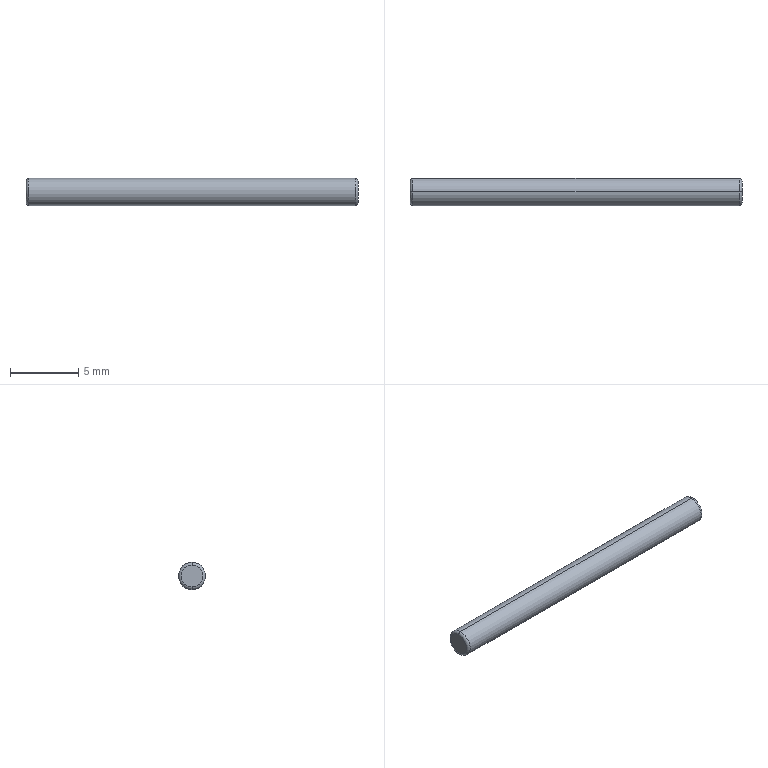Part | SolidWorks | features Extrusion 1, Fillet 1 | 1 solid | 8 faces | box 24.4 x 2 x 2 mm | volume 76.552 mm3 | torus 4 | cylinder 2 | plane 2 | commonest cylinder face diameters 2 x2
STEP:
#1=CARTESIAN_POINT('',(-12.2,0.,0.8));
#2=VERTEX_POINT('',#1);
#3=CARTESIAN_POINT('',(-12.2,0.,-0.8));
#4=VERTEX_POINT('',#3);
#5=CARTESIAN_POINT('',(-12.2,0.,0.));
#6=DIRECTION('',(-1.,0.,0.));
#7=DIRECTION('',(0.,0.,-1.));
#8=AXIS2_PLACEMENT_3D('',#5,#6,#7);
#9=CIRCLE('',#8,0.8);
#10=EDGE_CURVE('',#2,#4,#9,.T.);
#11=ORIENTED_EDGE('',*,*,#10,.F.);
#12=CARTESIAN_POINT('',(-12.,0.,1.));
#13=VERTEX_POINT('',#12);
#14=CARTESIAN_POINT('',(-12.,0.,0.8));
#15=DIRECTION('',(0.,1.,0.));
#16=DIRECTION('',(0.,0.,1.));
#17=AXIS2_PLACEMENT_3D('',#14,#15,#16);
#18=CIRCLE('',#17,0.2);
#19=EDGE_CURVE('',#2,#13,#18,.T.);
#20=ORIENTED_EDGE('',*,*,#19,.T.);
#21=CARTESIAN_POINT('',(-12.,0.,-1.));
#22=VERTEX_POINT('',#21);
#23=CARTESIAN_POINT('',(-12.,0.,0.));
#24=DIRECTION('',(1.,0.,0.));
#25=DIRECTION('',(0.,0.,-1.));
#26=AXIS2_PLACEMENT_3D('',#23,#24,#25);
#27=CIRCLE('',#26,1.);
#28=EDGE_CURVE('',#22,#13,#27,.T.);
#29=ORIENTED_EDGE('',*,*,#28,.F.);
#30=CARTESIAN_POINT('',(-12.,0.,-0.8));
#31=DIRECTION('',(0.,-1.,0.));
#32=DIRECTION('',(0.,0.,-1.));
#33=AXIS2_PLACEMENT_3D('',#30,#31,#32);
#34=CIRCLE('',#33,0.2);
#35=EDGE_CURVE('',#4,#22,#34,.T.);
#36=ORIENTED_EDGE('',*,*,#35,.F.);
#37=EDGE_LOOP('',(#11,#20,#29,#36));
#38=FACE_OUTER_BOUND('',#37,.T.);
#39=CARTESIAN_POINT('',(-12.,0.,0.));
#40=DIRECTION('',(1.,0.,0.));
#41=DIRECTION('',(0.,0.,-1.));
#42=AXIS2_PLACEMENT_3D('',#39,#40,#41);
#43=TOROIDAL_SURFACE('',#42,0.8,0.2);
#44=ADVANCED_FACE('',(#38),#43,.T.);
#45=CARTESIAN_POINT('',(12.,0.,1.));
#46=VERTEX_POINT('',#45);
#47=CARTESIAN_POINT('',(12.,0.,-1.));
#48=VERTEX_POINT('',#47);
#49=CARTESIAN_POINT('',(12.,0.,0.));
#50=DIRECTION('',(-1.,0.,0.));
#51=DIRECTION('',(0.,0.,-1.));
#52=AXIS2_PLACEMENT_3D('',#49,#50,#51);
#53=CIRCLE('',#52,1.);
#54=EDGE_CURVE('',#46,#48,#53,.T.);
#55=ORIENTED_EDGE('',*,*,#54,.F.);
#56=CARTESIAN_POINT('',(12.2,0.,0.8));
#57=VERTEX_POINT('',#56);
#58=CARTESIAN_POINT('',(12.,0.,0.8));
#59=DIRECTION('',(0.,1.,0.));
#60=DIRECTION('',(0.,0.,1.));
#61=AXIS2_PLACEMENT_3D('',#58,#59,#60);
#62=CIRCLE('',#61,0.2);
#63=EDGE_CURVE('',#46,#57,#62,.T.);
#64=ORIENTED_EDGE('',*,*,#63,.T.);
#65=CARTESIAN_POINT('',(12.2,0.,-0.8));
#66=VERTEX_POINT('',#65);
#67=CARTESIAN_POINT('',(12.2,0.,0.));
#68=DIRECTION('',(1.,0.,0.));
#69=DIRECTION('',(0.,0.,-1.));
#70=AXIS2_PLACEMENT_3D('',#67,#68,#69);
#71=CIRCLE('',#70,0.8);
#72=EDGE_CURVE('',#66,#57,#71,.T.);
#73=ORIENTED_EDGE('',*,*,#72,.F.);
#74=CARTESIAN_POINT('',(12.,0.,-0.8));
#75=DIRECTION('',(0.,-1.,0.));
#76=DIRECTION('',(0.,0.,-1.));
#77=AXIS2_PLACEMENT_3D('',#74,#75,#76);
#78=CIRCLE('',#77,0.2);
#79=EDGE_CURVE('',#48,#66,#78,.T.);
#80=ORIENTED_EDGE('',*,*,#79,.F.);
#81=EDGE_LOOP('',(#55,#64,#73,#80));
#82=FACE_OUTER_BOUND('',#81,.T.);
#83=CARTESIAN_POINT('',(12.,0.,0.));
#84=DIRECTION('',(1.,0.,0.));
#85=DIRECTION('',(0.,0.,-1.));
#86=AXIS2_PLACEMENT_3D('',#83,#84,#85);
#87=TOROIDAL_SURFACE('',#86,0.8,0.2);
#88=ADVANCED_FACE('',(#82),#87,.T.);
#89=ORIENTED_EDGE('',*,*,#54,.T.);
#90=CARTESIAN_POINT('',(12.2,0.,-1.));
#91=DIRECTION('',(-1.,0.,0.));
#92=VECTOR('',#91,1000.);
#93=LINE('',#90,#92);
#94=EDGE_CURVE('',#48,#22,#93,.T.);
#95=ORIENTED_EDGE('',*,*,#94,.T.);
#96=ORIENTED_EDGE('',*,*,#28,.T.);
#97=CARTESIAN_POINT('',(12.2,0.,1.));
#98=DIRECTION('',(-1.,0.,0.));
#99=VECTOR('',#98,1000.);
#100=LINE('',#97,#99);
#101=EDGE_CURVE('',#46,#13,#100,.T.);
#102=ORIENTED_EDGE('',*,*,#101,.F.);
#103=EDGE_LOOP('',(#89,#95,#96,#102));
#104=FACE_OUTER_BOUND('',#103,.T.);
#105=CARTESIAN_POINT('',(12.2,0.,0.));
#106=DIRECTION('',(-1.,0.,0.));
#107=DIRECTION('',(0.,0.,1.));
#108=AXIS2_PLACEMENT_3D('',#105,#106,#107);
#109=CYLINDRICAL_SURFACE('',#108,1.);
#110=ADVANCED_FACE('',(#104),#109,.T.);
#111=ORIENTED_EDGE('',*,*,#94,.F.);
#112=CARTESIAN_POINT('',(12.,0.,0.));
#113=DIRECTION('',(-1.,0.,0.));
#114=DIRECTION('',(0.,0.,-1.));
#115=AXIS2_PLACEMENT_3D('',#112,#113,#114);
#116=CIRCLE('',#115,1.);
#117=EDGE_CURVE('',#48,#46,#116,.T.);
#118=ORIENTED_EDGE('',*,*,#117,.T.);
#119=ORIENTED_EDGE('',*,*,#101,.T.);
#120=CARTESIAN_POINT('',(-12.,0.,0.));
#121=DIRECTION('',(1.,0.,0.));
#122=DIRECTION('',(0.,0.,-1.));
#123=AXIS2_PLACEMENT_3D('',#120,#121,#122);
#124=CIRCLE('',#123,1.);
#125=EDGE_CURVE('',#13,#22,#124,.T.);
#126=ORIENTED_EDGE('',*,*,#125,.T.);
#127=EDGE_LOOP('',(#111,#118,#119,#126));
#128=FACE_OUTER_BOUND('',#127,.T.);
#129=CARTESIAN_POINT('',(12.2,0.,0.));
#130=DIRECTION('',(-1.,0.,0.));
#131=DIRECTION('',(0.,0.,1.));
#132=AXIS2_PLACEMENT_3D('',#129,#130,#131);
#133=CYLINDRICAL_SURFACE('',#132,1.);
#134=ADVANCED_FACE('',(#128),#133,.T.);
#135=ORIENTED_EDGE('',*,*,#72,.T.);
#136=CARTESIAN_POINT('',(12.2,0.,0.));
#137=DIRECTION('',(1.,0.,0.));
#138=DIRECTION('',(0.,0.,-1.));
#139=AXIS2_PLACEMENT_3D('',#136,#137,#138);
#140=CIRCLE('',#139,0.8);
#141=EDGE_CURVE('',#57,#66,#140,.T.);
#142=ORIENTED_EDGE('',*,*,#141,.T.);
#143=EDGE_LOOP('',(#135,#142));
#144=FACE_OUTER_BOUND('',#143,.T.);
#145=CARTESIAN_POINT('',(12.2,0.,0.));
#146=DIRECTION('',(1.,0.,0.));
#147=DIRECTION('',(0.,0.,-1.));
#148=AXIS2_PLACEMENT_3D('',#145,#146,#147);
#149=PLANE('',#148);
#150=ADVANCED_FACE('',(#144),#149,.T.);
#151=CARTESIAN_POINT('',(-12.2,0.,0.));
#152=DIRECTION('',(-1.,0.,0.));
#153=DIRECTION('',(0.,0.,-1.));
#154=AXIS2_PLACEMENT_3D('',#151,#152,#153);
#155=CIRCLE('',#154,0.8);
#156=EDGE_CURVE('',#4,#2,#155,.T.);
#157=ORIENTED_EDGE('',*,*,#156,.T.);
#158=ORIENTED_EDGE('',*,*,#10,.T.);
#159=EDGE_LOOP('',(#157,#158));
#160=FACE_OUTER_BOUND('',#159,.T.);
#161=CARTESIAN_POINT('',(-12.2,0.,0.));
#162=DIRECTION('',(1.,0.,0.));
#163=DIRECTION('',(0.,0.,-1.));
#164=AXIS2_PLACEMENT_3D('',#161,#162,#163);
#165=PLANE('',#164);
#166=ADVANCED_FACE('',(#160),#165,.F.);
#167=ORIENTED_EDGE('',*,*,#63,.F.);
#168=ORIENTED_EDGE('',*,*,#117,.F.);
#169=ORIENTED_EDGE('',*,*,#79,.T.);
#170=ORIENTED_EDGE('',*,*,#141,.F.);
#171=EDGE_LOOP('',(#167,#168,#169,#170));
#172=FACE_OUTER_BOUND('',#171,.T.);
#173=CARTESIAN_POINT('',(12.,0.,0.));
#174=DIRECTION('',(1.,0.,0.));
#175=DIRECTION('',(0.,0.,-1.));
#176=AXIS2_PLACEMENT_3D('',#173,#174,#175);
#177=TOROIDAL_SURFACE('',#176,0.8,0.2);
#178=ADVANCED_FACE('',(#172),#177,.T.);
#179=ORIENTED_EDGE('',*,*,#19,.F.);
#180=ORIENTED_EDGE('',*,*,#156,.F.);
#181=ORIENTED_EDGE('',*,*,#35,.T.);
#182=ORIENTED_EDGE('',*,*,#125,.F.);
#183=EDGE_LOOP('',(#179,#180,#181,#182));
#184=FACE_OUTER_BOUND('',#183,.T.);
#185=CARTESIAN_POINT('',(-12.,0.,0.));
#186=DIRECTION('',(1.,0.,0.));
#187=DIRECTION('',(0.,0.,-1.));
#188=AXIS2_PLACEMENT_3D('',#185,#186,#187);
#189=TOROIDAL_SURFACE('',#188,0.8,0.2);
#190=ADVANCED_FACE('',(#184),#189,.T.);
#191=CLOSED_SHELL('',(#44,#88,#110,#134,#150,#166,#178,#190));
#192=MANIFOLD_SOLID_BREP('',#191);
#193=CARTESIAN_POINT('',(0.,0.,0.));
#194=DIRECTION('',(0.,0.,1.));
#195=DIRECTION('',(1.,0.,0.));
#196=AXIS2_PLACEMENT_3D('',#193,#194,#195);
#197=(LENGTH_UNIT()NAMED_UNIT(*)SI_UNIT(.MILLI.,.METRE.));
#198=UNCERTAINTY_MEASURE_WITH_UNIT(LENGTH_MEASURE(0.00001),#197,'','');
#199=(NAMED_UNIT(*)PLANE_ANGLE_UNIT()SI_UNIT($,.RADIAN.));
#200=(NAMED_UNIT(*)SI_UNIT($,.STERADIAN.)SOLID_ANGLE_UNIT());
#201=(GEOMETRIC_REPRESENTATION_CONTEXT(3)GLOBAL_UNCERTAINTY_ASSIGNED_CONTEXT((#198))GLOBAL_UNIT_ASSIGNED_CONTEXT((#197,#199,#200))REPRESENTATION_CONTEXT('',''));
#202=ADVANCED_BREP_SHAPE_REPRESENTATION('',(#192,#196),#201);